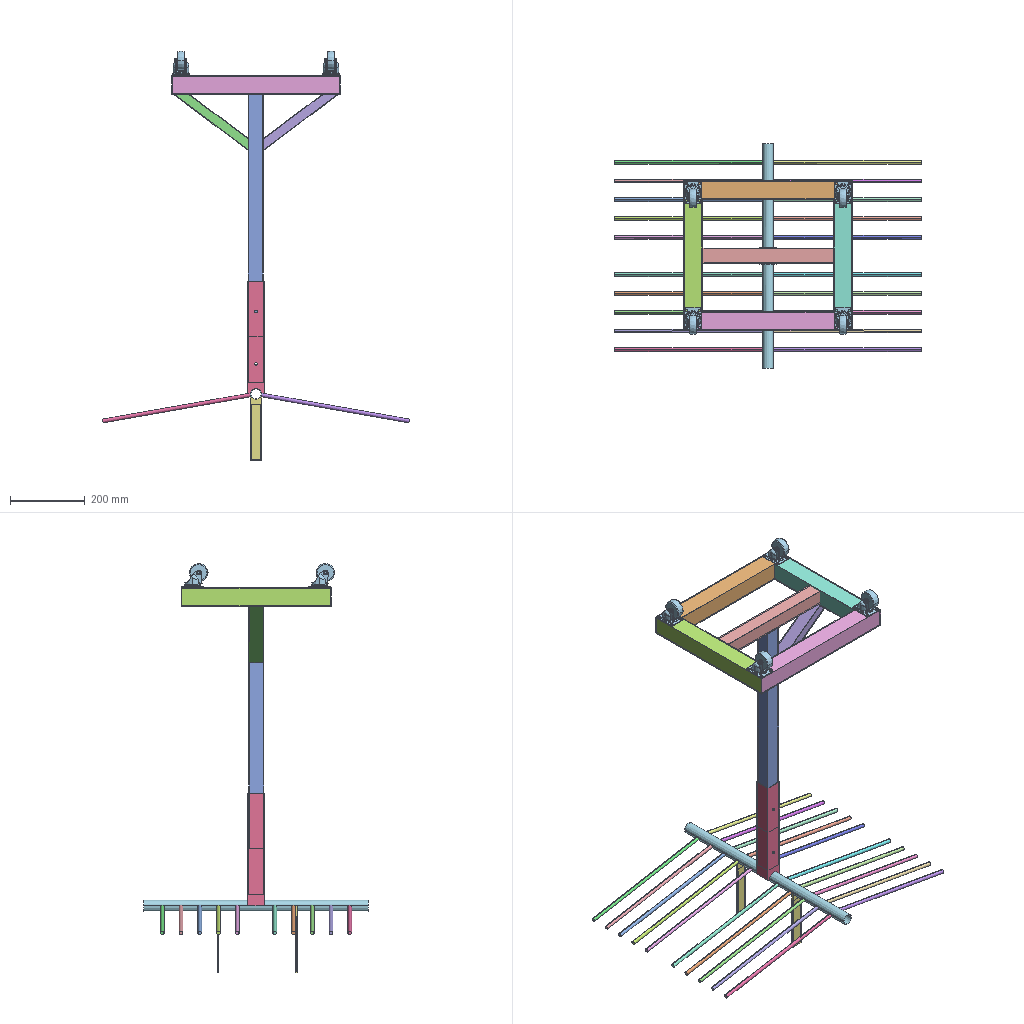Assembly | SolidWorks | 5 different items | 9 placed | box 819 x 600 x 1092 mm
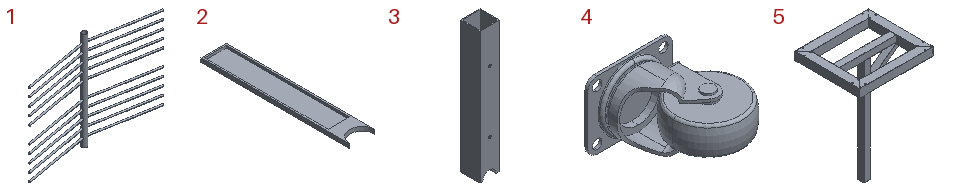Parts list (item | quantity | size | volume | features):
1 | x1 | 819.127 x 91.988 x 600 mm | 708781 mm3 | features ICE 4, Extrusion 1
2 | x2 | 30 x 178 x 5 mm | 13389 mm3 | features ICE 4, Extrusion 1
3 | x1 | 43.5 x 43.5 x 300 mm | 108012 mm3 | features ICE 3, Extrusion 1, HoleWzd 1
4 | x4 | 70.5 x 65 x 47 mm | 52288 mm3 | features BaseBody 1
5 | x1 | 450 x 400 x 695 mm | 762729 mm3 | features Shell 8, Gusset 2, ICE 2, WeldMemberFeat 2, HoleWzd 1, WeldmentFeature 1
Mates (type | each side: item.copy, entity, surface, feature):
Coincident | 5.1 face plane Boss-Extrude2 | 3.1 face plane Boss-Extrude1 | 2 times
Coincident | 5.1 face plane Square bar SQUARE BAR 50(17) | 4.1 face plane Input1
Concentric | 5.1 face cylinder M6 Tapped Hole1 | 4.1 face cylinder Input1 | 4 times
Coincident | 5.1 face plane Square bar SQUARE BAR 50(17) | 4.2 face plane Input1
Coincident | 5.1 face plane Square bar SQUARE BAR 50(17) | 4.3 face plane Input1
Coincident | 5.1 face plane Square bar SQUARE BAR 50(17) | 4.4 face plane Input1
Concentric | 5.1 face cylinder M6 Tapped Hole1 | 4.2 face cylinder Input1 | 4 times
Concentric | 5.1 face cylinder M6 Tapped Hole1 | 4.3 face cylinder Input1 | 4 times
Concentric | 5.1 face cylinder M6 Tapped Hole1 | 4.4 face cylinder Input1 | 3 times
Concentric | 5.1 edge | 4.4 face cylinder Input1
Concentric | 3.1 face cylinder Cut-Extrude1 | 1.1 face cylinder Boss-Extrude1
Concentric | 3.1 face cylinder Cut-Extrude2 | 1.1 face cylinder Cut-Extrude1
Concentric | 1.1 face cylinder Boss-Extrude1 | 2.1 face cylinder Cut-Extrude3
Parallel | 5.1 face plane Square bar SQUARE BAR 50(17) | 2.1 face plane Boss-Extrude1
Concentric | 1.1 face cylinder Boss-Extrude1 | 2.2 face cylinder Cut-Extrude3
DistanceDim | 2.2 face plane Cut-Extrude1 | 2.1 face plane Cut-Extrude1
Parallel | 3.1 face plane Boss-Extrude1 | 2.2 face plane Boss-Extrude1
Parallel | 3.1 face plane Boss-Extrude1 | 1.1 select_type:24
Parallel | 3.1 face plane Boss-Extrude1 | 2.1 face plane Boss-Extrude1 | 2 times
DistanceDim | 2.1 face plane Boss-Extrude1 | 1.1 face plane Boss-Extrude1